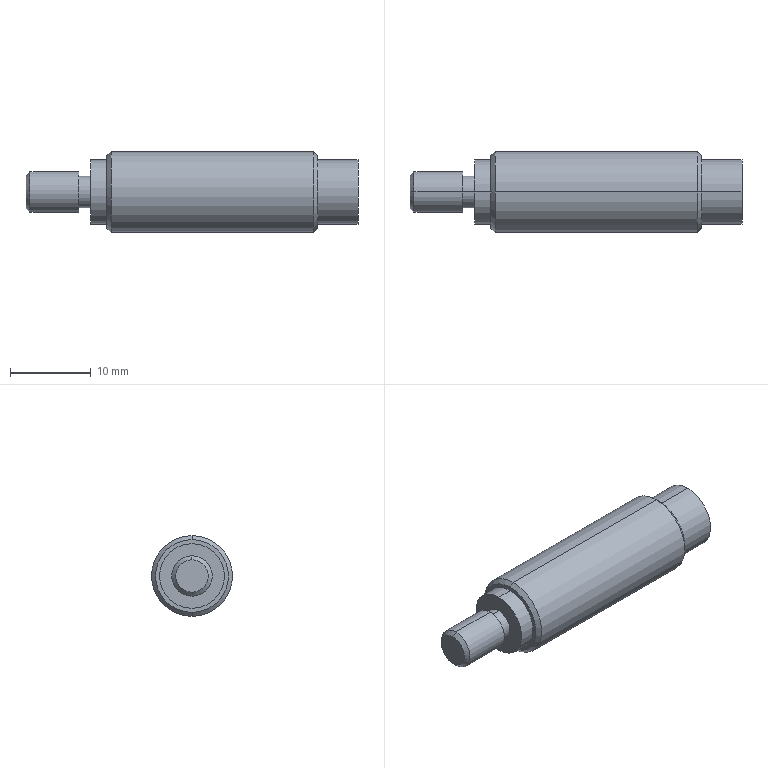Part | STEP file | 0232_009_SETK10-26-M5-N4 | 1 solid | 28 faces | box 41 x 10 x 10 mm | volume 2435 mm3 | cylinder 12 | cone 10 | plane 6 | commonest cylinder face diameters 8 x4 3.242 x2 3.9 x2 5 x2 10 x2